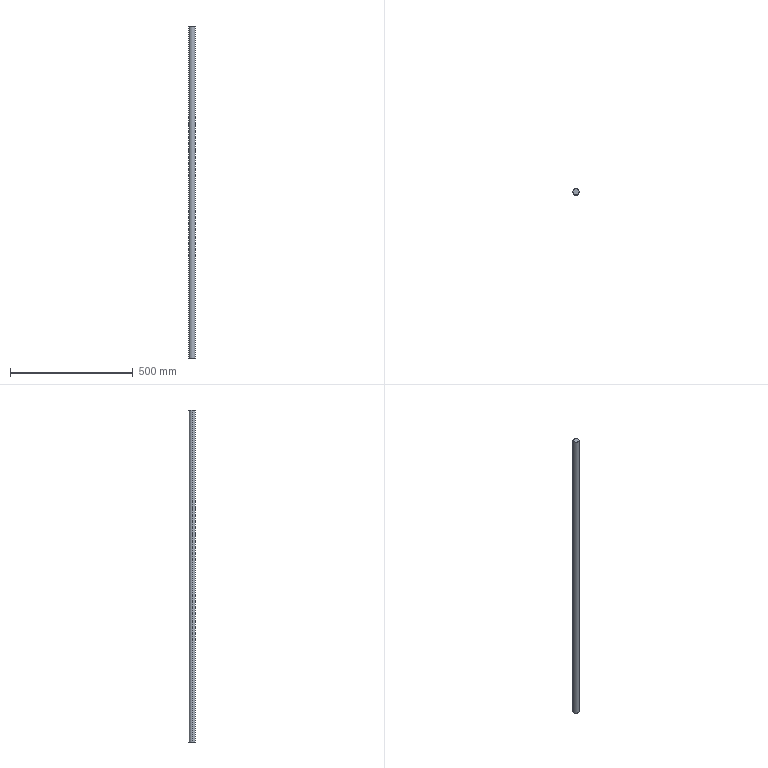Part | SolidWorks | features Extrusion 1 | 1 solid | 4 faces | box 25 x 25 x 1352 mm | volume 663661 mm3 | cylinder 2 | plane 2 | commonest cylinder face diameters 25 x2
STEP:
#1=CARTESIAN_POINT('',(12.5,0.,1352.));
#2=VERTEX_POINT('',#1);
#3=CARTESIAN_POINT('',(-12.5,0.,1352.));
#4=VERTEX_POINT('',#3);
#5=CARTESIAN_POINT('',(0.,0.,1352.));
#6=DIRECTION('',(0.,0.,1.));
#7=DIRECTION('',(1.,0.,0.));
#8=AXIS2_PLACEMENT_3D('',#5,#6,#7);
#9=CIRCLE('',#8,12.5);
#10=EDGE_CURVE('',#2,#4,#9,.T.);
#11=ORIENTED_EDGE('',*,*,#10,.F.);
#12=CARTESIAN_POINT('',(12.5,0.,0.));
#13=VERTEX_POINT('',#12);
#14=CARTESIAN_POINT('',(12.5,0.,1352.));
#15=DIRECTION('',(0.,0.,-1.));
#16=VECTOR('',#15,1000.);
#17=LINE('',#14,#16);
#18=EDGE_CURVE('',#2,#13,#17,.T.);
#19=ORIENTED_EDGE('',*,*,#18,.T.);
#20=CARTESIAN_POINT('',(-12.5,0.,0.));
#21=VERTEX_POINT('',#20);
#22=CARTESIAN_POINT('',(0.,0.,0.));
#23=DIRECTION('',(0.,0.,1.));
#24=DIRECTION('',(1.,0.,0.));
#25=AXIS2_PLACEMENT_3D('',#22,#23,#24);
#26=CIRCLE('',#25,12.5);
#27=EDGE_CURVE('',#13,#21,#26,.T.);
#28=ORIENTED_EDGE('',*,*,#27,.T.);
#29=CARTESIAN_POINT('',(-12.5,0.,1352.));
#30=DIRECTION('',(0.,0.,-1.));
#31=VECTOR('',#30,1000.);
#32=LINE('',#29,#31);
#33=EDGE_CURVE('',#4,#21,#32,.T.);
#34=ORIENTED_EDGE('',*,*,#33,.F.);
#35=EDGE_LOOP('',(#11,#19,#28,#34));
#36=FACE_OUTER_BOUND('',#35,.T.);
#37=CARTESIAN_POINT('',(0.,0.,1352.));
#38=DIRECTION('',(0.,0.,-1.));
#39=DIRECTION('',(-1.,0.,0.));
#40=AXIS2_PLACEMENT_3D('',#37,#38,#39);
#41=CYLINDRICAL_SURFACE('',#40,12.5);
#42=ADVANCED_FACE('',(#36),#41,.T.);
#43=ORIENTED_EDGE('',*,*,#18,.F.);
#44=CARTESIAN_POINT('',(0.,0.,1352.));
#45=DIRECTION('',(0.,0.,1.));
#46=DIRECTION('',(1.,0.,0.));
#47=AXIS2_PLACEMENT_3D('',#44,#45,#46);
#48=CIRCLE('',#47,12.5);
#49=EDGE_CURVE('',#4,#2,#48,.T.);
#50=ORIENTED_EDGE('',*,*,#49,.F.);
#51=ORIENTED_EDGE('',*,*,#33,.T.);
#52=CARTESIAN_POINT('',(0.,0.,0.));
#53=DIRECTION('',(0.,0.,1.));
#54=DIRECTION('',(1.,0.,0.));
#55=AXIS2_PLACEMENT_3D('',#52,#53,#54);
#56=CIRCLE('',#55,12.5);
#57=EDGE_CURVE('',#21,#13,#56,.T.);
#58=ORIENTED_EDGE('',*,*,#57,.T.);
#59=EDGE_LOOP('',(#43,#50,#51,#58));
#60=FACE_OUTER_BOUND('',#59,.T.);
#61=CARTESIAN_POINT('',(0.,0.,1352.));
#62=DIRECTION('',(0.,0.,-1.));
#63=DIRECTION('',(-1.,0.,0.));
#64=AXIS2_PLACEMENT_3D('',#61,#62,#63);
#65=CYLINDRICAL_SURFACE('',#64,12.5);
#66=ADVANCED_FACE('',(#60),#65,.T.);
#67=ORIENTED_EDGE('',*,*,#49,.T.);
#68=ORIENTED_EDGE('',*,*,#10,.T.);
#69=EDGE_LOOP('',(#67,#68));
#70=FACE_OUTER_BOUND('',#69,.T.);
#71=CARTESIAN_POINT('',(0.,0.,1352.));
#72=DIRECTION('',(0.,0.,1.));
#73=DIRECTION('',(1.,0.,0.));
#74=AXIS2_PLACEMENT_3D('',#71,#72,#73);
#75=PLANE('',#74);
#76=ADVANCED_FACE('',(#70),#75,.T.);
#77=ORIENTED_EDGE('',*,*,#57,.F.);
#78=ORIENTED_EDGE('',*,*,#27,.F.);
#79=EDGE_LOOP('',(#77,#78));
#80=FACE_OUTER_BOUND('',#79,.T.);
#81=CARTESIAN_POINT('',(0.,0.,0.));
#82=DIRECTION('',(0.,0.,1.));
#83=DIRECTION('',(1.,0.,0.));
#84=AXIS2_PLACEMENT_3D('',#81,#82,#83);
#85=PLANE('',#84);
#86=ADVANCED_FACE('',(#80),#85,.F.);
#87=CLOSED_SHELL('',(#42,#66,#76,#86));
#88=MANIFOLD_SOLID_BREP('',#87);
#89=CARTESIAN_POINT('',(0.,0.,0.));
#90=DIRECTION('',(0.,0.,1.));
#91=DIRECTION('',(1.,0.,0.));
#92=AXIS2_PLACEMENT_3D('',#89,#90,#91);
#93=(LENGTH_UNIT()NAMED_UNIT(*)SI_UNIT(.MILLI.,.METRE.));
#94=UNCERTAINTY_MEASURE_WITH_UNIT(LENGTH_MEASURE(0.00001),#93,'','');
#95=(NAMED_UNIT(*)PLANE_ANGLE_UNIT()SI_UNIT($,.RADIAN.));
#96=(NAMED_UNIT(*)SI_UNIT($,.STERADIAN.)SOLID_ANGLE_UNIT());
#97=(GEOMETRIC_REPRESENTATION_CONTEXT(3)GLOBAL_UNCERTAINTY_ASSIGNED_CONTEXT((#94))GLOBAL_UNIT_ASSIGNED_CONTEXT((#93,#95,#96))REPRESENTATION_CONTEXT('',''));
#98=ADVANCED_BREP_SHAPE_REPRESENTATION('',(#88,#92),#97);